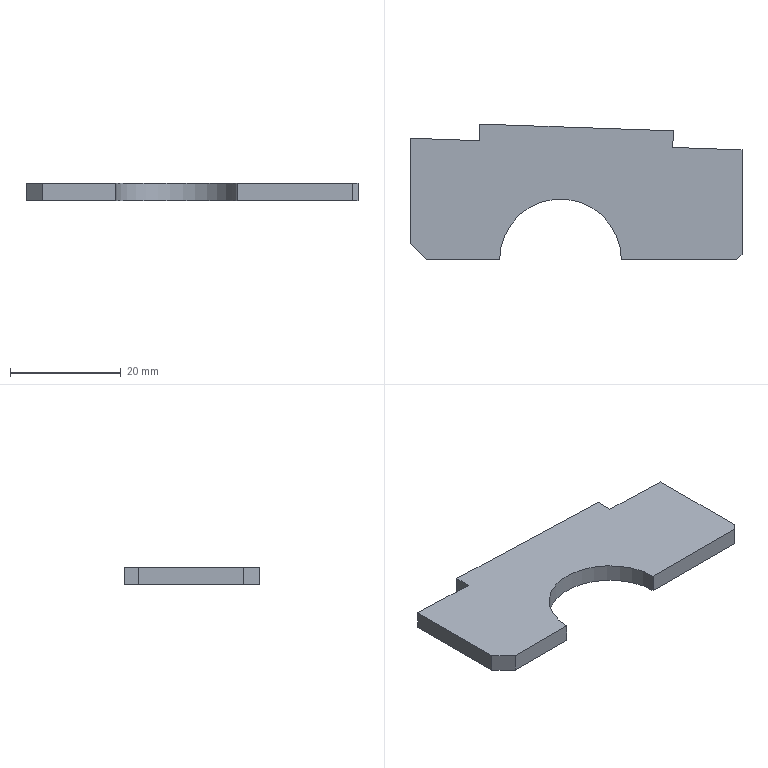Part | SolidWorks | features FlatPattern 1, SMBaseFlange 1, SheetMetal 1 | 1 solid | 14 faces | box 60 x 24.545 x 3.2 mm | volume 3731 mm3 | plane 13 | cylinder 1 | commonest cylinder face diameters 22 x1
STEP:
#1=CARTESIAN_POINT('',(-504.444,-212.712,0.));
#2=VERTEX_POINT('',#1);
#3=CARTESIAN_POINT('',(-501.444,-215.712,0.));
#4=VERTEX_POINT('',#3);
#5=CARTESIAN_POINT('',(-504.444,-212.712,0.));
#6=DIRECTION('',(0.7071,-0.7071,0.));
#7=VECTOR('',#6,1000.);
#8=LINE('',#5,#7);
#9=EDGE_CURVE('',#2,#4,#8,.T.);
#10=ORIENTED_EDGE('',*,*,#9,.T.);
#11=CARTESIAN_POINT('',(-501.444,-215.712,3.2));
#12=VERTEX_POINT('',#11);
#13=CARTESIAN_POINT('',(-501.444,-215.712,3.2));
#14=DIRECTION('',(0.,0.,-1.));
#15=VECTOR('',#14,1000.);
#16=LINE('',#13,#15);
#17=EDGE_CURVE('',#12,#4,#16,.T.);
#18=ORIENTED_EDGE('',*,*,#17,.F.);
#19=CARTESIAN_POINT('',(-504.444,-212.712,3.2));
#20=VERTEX_POINT('',#19);
#21=CARTESIAN_POINT('',(-504.444,-212.712,3.2));
#22=DIRECTION('',(0.7071,-0.7071,0.));
#23=VECTOR('',#22,1000.);
#24=LINE('',#21,#23);
#25=EDGE_CURVE('',#20,#12,#24,.T.);
#26=ORIENTED_EDGE('',*,*,#25,.F.);
#27=CARTESIAN_POINT('',(-504.444,-212.712,3.2));
#28=DIRECTION('',(0.,0.,-1.));
#29=VECTOR('',#28,1000.);
#30=LINE('',#27,#29);
#31=EDGE_CURVE('',#20,#2,#30,.T.);
#32=ORIENTED_EDGE('',*,*,#31,.T.);
#33=EDGE_LOOP('',(#10,#18,#26,#32));
#34=FACE_OUTER_BOUND('',#33,.T.);
#35=CARTESIAN_POINT('',(-504.444,-212.712,3.2));
#36=DIRECTION('',(0.7071,0.7071,0.));
#37=DIRECTION('',(-0.7071,0.7071,0.));
#38=AXIS2_PLACEMENT_3D('',#35,#36,#37);
#39=PLANE('',#38);
#40=ADVANCED_FACE('',(#34),#39,.F.);
#41=CARTESIAN_POINT('',(-488.244,-215.712,0.));
#42=VERTEX_POINT('',#41);
#43=CARTESIAN_POINT('',(-501.444,-215.712,0.));
#44=DIRECTION('',(1.,0.,0.));
#45=VECTOR('',#44,1000.);
#46=LINE('',#43,#45);
#47=EDGE_CURVE('',#4,#42,#46,.T.);
#48=ORIENTED_EDGE('',*,*,#47,.T.);
#49=CARTESIAN_POINT('',(-488.244,-215.712,3.2));
#50=VERTEX_POINT('',#49);
#51=CARTESIAN_POINT('',(-488.244,-215.712,3.2));
#52=DIRECTION('',(0.,0.,-1.));
#53=VECTOR('',#52,1000.);
#54=LINE('',#51,#53);
#55=EDGE_CURVE('',#50,#42,#54,.T.);
#56=ORIENTED_EDGE('',*,*,#55,.F.);
#57=CARTESIAN_POINT('',(-501.444,-215.712,3.2));
#58=DIRECTION('',(1.,0.,0.));
#59=VECTOR('',#58,1000.);
#60=LINE('',#57,#59);
#61=EDGE_CURVE('',#12,#50,#60,.T.);
#62=ORIENTED_EDGE('',*,*,#61,.F.);
#63=ORIENTED_EDGE('',*,*,#17,.T.);
#64=EDGE_LOOP('',(#48,#56,#62,#63));
#65=FACE_OUTER_BOUND('',#64,.T.);
#66=CARTESIAN_POINT('',(-501.444,-215.712,3.2));
#67=DIRECTION('',(0.,1.,0.));
#68=DIRECTION('',(0.,0.,1.));
#69=AXIS2_PLACEMENT_3D('',#66,#67,#68);
#70=PLANE('',#69);
#71=ADVANCED_FACE('',(#65),#70,.F.);
#72=CARTESIAN_POINT('',(-466.244,-215.712,0.));
#73=VERTEX_POINT('',#72);
#74=CARTESIAN_POINT('',(-477.244,-215.712,0.));
#75=DIRECTION('',(0.,0.,-1.));
#76=DIRECTION('',(1.,0.,0.));
#77=AXIS2_PLACEMENT_3D('',#74,#75,#76);
#78=CIRCLE('',#77,11.);
#79=EDGE_CURVE('',#42,#73,#78,.T.);
#80=ORIENTED_EDGE('',*,*,#79,.T.);
#81=CARTESIAN_POINT('',(-466.244,-215.712,3.2));
#82=VERTEX_POINT('',#81);
#83=CARTESIAN_POINT('',(-466.244,-215.712,3.2));
#84=DIRECTION('',(0.,0.,-1.));
#85=VECTOR('',#84,1000.);
#86=LINE('',#83,#85);
#87=EDGE_CURVE('',#82,#73,#86,.T.);
#88=ORIENTED_EDGE('',*,*,#87,.F.);
#89=CARTESIAN_POINT('',(-477.244,-215.712,3.2));
#90=DIRECTION('',(0.,0.,-1.));
#91=DIRECTION('',(1.,0.,0.));
#92=AXIS2_PLACEMENT_3D('',#89,#90,#91);
#93=CIRCLE('',#92,11.);
#94=EDGE_CURVE('',#50,#82,#93,.T.);
#95=ORIENTED_EDGE('',*,*,#94,.F.);
#96=ORIENTED_EDGE('',*,*,#55,.T.);
#97=EDGE_LOOP('',(#80,#88,#95,#96));
#98=FACE_OUTER_BOUND('',#97,.T.);
#99=CARTESIAN_POINT('',(-477.244,-215.712,3.2));
#100=DIRECTION('',(0.,0.,-1.));
#101=DIRECTION('',(-1.,0.,0.));
#102=AXIS2_PLACEMENT_3D('',#99,#100,#101);
#103=CYLINDRICAL_SURFACE('',#102,11.);
#104=ADVANCED_FACE('',(#98),#103,.F.);
#105=CARTESIAN_POINT('',(-445.444,-215.712,0.));
#106=VERTEX_POINT('',#105);
#107=CARTESIAN_POINT('',(-466.244,-215.712,0.));
#108=DIRECTION('',(1.,0.,0.));
#109=VECTOR('',#108,1000.);
#110=LINE('',#107,#109);
#111=EDGE_CURVE('',#73,#106,#110,.T.);
#112=ORIENTED_EDGE('',*,*,#111,.T.);
#113=CARTESIAN_POINT('',(-445.444,-215.712,3.2));
#114=VERTEX_POINT('',#113);
#115=CARTESIAN_POINT('',(-445.444,-215.712,3.2));
#116=DIRECTION('',(0.,0.,-1.));
#117=VECTOR('',#116,1000.);
#118=LINE('',#115,#117);
#119=EDGE_CURVE('',#114,#106,#118,.T.);
#120=ORIENTED_EDGE('',*,*,#119,.F.);
#121=CARTESIAN_POINT('',(-466.244,-215.712,3.2));
#122=DIRECTION('',(1.,0.,0.));
#123=VECTOR('',#122,1000.);
#124=LINE('',#121,#123);
#125=EDGE_CURVE('',#82,#114,#124,.T.);
#126=ORIENTED_EDGE('',*,*,#125,.F.);
#127=ORIENTED_EDGE('',*,*,#87,.T.);
#128=EDGE_LOOP('',(#112,#120,#126,#127));
#129=FACE_OUTER_BOUND('',#128,.T.);
#130=CARTESIAN_POINT('',(-466.244,-215.712,3.2));
#131=DIRECTION('',(0.,1.,0.));
#132=DIRECTION('',(0.,0.,1.));
#133=AXIS2_PLACEMENT_3D('',#130,#131,#132);
#134=PLANE('',#133);
#135=ADVANCED_FACE('',(#129),#134,.F.);
#136=CARTESIAN_POINT('',(-444.444,-214.712,0.));
#137=VERTEX_POINT('',#136);
#138=CARTESIAN_POINT('',(-445.444,-215.712,0.));
#139=DIRECTION('',(0.7071,0.7071,0.));
#140=VECTOR('',#139,1000.);
#141=LINE('',#138,#140);
#142=EDGE_CURVE('',#106,#137,#141,.T.);
#143=ORIENTED_EDGE('',*,*,#142,.T.);
#144=CARTESIAN_POINT('',(-444.444,-214.712,3.2));
#145=VERTEX_POINT('',#144);
#146=CARTESIAN_POINT('',(-444.444,-214.712,3.2));
#147=DIRECTION('',(0.,0.,-1.));
#148=VECTOR('',#147,1000.);
#149=LINE('',#146,#148);
#150=EDGE_CURVE('',#145,#137,#149,.T.);
#151=ORIENTED_EDGE('',*,*,#150,.F.);
#152=CARTESIAN_POINT('',(-445.444,-215.712,3.2));
#153=DIRECTION('',(0.7071,0.7071,0.));
#154=VECTOR('',#153,1000.);
#155=LINE('',#152,#154);
#156=EDGE_CURVE('',#114,#145,#155,.T.);
#157=ORIENTED_EDGE('',*,*,#156,.F.);
#158=ORIENTED_EDGE('',*,*,#119,.T.);
#159=EDGE_LOOP('',(#143,#151,#157,#158));
#160=FACE_OUTER_BOUND('',#159,.T.);
#161=CARTESIAN_POINT('',(-445.444,-215.712,3.2));
#162=DIRECTION('',(-0.7071,0.7071,0.));
#163=DIRECTION('',(-0.7071,-0.7071,0.));
#164=AXIS2_PLACEMENT_3D('',#161,#162,#163);
#165=PLANE('',#164);
#166=ADVANCED_FACE('',(#160),#165,.F.);
#167=CARTESIAN_POINT('',(-444.444,-195.825,0.));
#168=VERTEX_POINT('',#167);
#169=CARTESIAN_POINT('',(-444.444,-214.712,0.));
#170=DIRECTION('',(0.,1.,0.));
#171=VECTOR('',#170,1000.);
#172=LINE('',#169,#171);
#173=EDGE_CURVE('',#137,#168,#172,.T.);
#174=ORIENTED_EDGE('',*,*,#173,.T.);
#175=CARTESIAN_POINT('',(-444.444,-195.825,3.2));
#176=VERTEX_POINT('',#175);
#177=CARTESIAN_POINT('',(-444.444,-195.825,3.2));
#178=DIRECTION('',(0.,0.,-1.));
#179=VECTOR('',#178,1000.);
#180=LINE('',#177,#179);
#181=EDGE_CURVE('',#176,#168,#180,.T.);
#182=ORIENTED_EDGE('',*,*,#181,.F.);
#183=CARTESIAN_POINT('',(-444.444,-214.712,3.2));
#184=DIRECTION('',(0.,1.,0.));
#185=VECTOR('',#184,1000.);
#186=LINE('',#183,#185);
#187=EDGE_CURVE('',#145,#176,#186,.T.);
#188=ORIENTED_EDGE('',*,*,#187,.F.);
#189=ORIENTED_EDGE('',*,*,#150,.T.);
#190=EDGE_LOOP('',(#174,#182,#188,#189));
#191=FACE_OUTER_BOUND('',#190,.T.);
#192=CARTESIAN_POINT('',(-444.444,-214.712,3.2));
#193=DIRECTION('',(-1.,0.,0.));
#194=DIRECTION('',(0.,0.,1.));
#195=AXIS2_PLACEMENT_3D('',#192,#193,#194);
#196=PLANE('',#195);
#197=ADVANCED_FACE('',(#191),#196,.F.);
#198=CARTESIAN_POINT('',(-456.954,-195.388,0.));
#199=VERTEX_POINT('',#198);
#200=CARTESIAN_POINT('',(-444.444,-195.825,0.));
#201=DIRECTION('',(-0.9994,0.0349,0.));
#202=VECTOR('',#201,1000.);
#203=LINE('',#200,#202);
#204=EDGE_CURVE('',#168,#199,#203,.T.);
#205=ORIENTED_EDGE('',*,*,#204,.T.);
#206=CARTESIAN_POINT('',(-456.954,-195.388,3.2));
#207=VERTEX_POINT('',#206);
#208=CARTESIAN_POINT('',(-456.954,-195.388,3.2));
#209=DIRECTION('',(0.,0.,-1.));
#210=VECTOR('',#209,1000.);
#211=LINE('',#208,#210);
#212=EDGE_CURVE('',#207,#199,#211,.T.);
#213=ORIENTED_EDGE('',*,*,#212,.F.);
#214=CARTESIAN_POINT('',(-444.444,-195.825,3.2));
#215=DIRECTION('',(-0.9994,0.0349,0.));
#216=VECTOR('',#215,1000.);
#217=LINE('',#214,#216);
#218=EDGE_CURVE('',#176,#207,#217,.T.);
#219=ORIENTED_EDGE('',*,*,#218,.F.);
#220=ORIENTED_EDGE('',*,*,#181,.T.);
#221=EDGE_LOOP('',(#205,#213,#219,#220));
#222=FACE_OUTER_BOUND('',#221,.T.);
#223=CARTESIAN_POINT('',(-444.444,-195.825,3.2));
#224=DIRECTION('',(-0.0349,-0.9994,0.));
#225=DIRECTION('',(0.9994,-0.0349,0.));
#226=AXIS2_PLACEMENT_3D('',#223,#224,#225);
#227=PLANE('',#226);
#228=ADVANCED_FACE('',(#222),#227,.F.);
#229=CARTESIAN_POINT('',(-456.85,-192.388,0.));
#230=VERTEX_POINT('',#229);
#231=CARTESIAN_POINT('',(-456.954,-195.388,0.));
#232=DIRECTION('',(0.0349,0.9994,0.));
#233=VECTOR('',#232,1000.);
#234=LINE('',#231,#233);
#235=EDGE_CURVE('',#199,#230,#234,.T.);
#236=ORIENTED_EDGE('',*,*,#235,.T.);
#237=CARTESIAN_POINT('',(-456.85,-192.388,3.2));
#238=VERTEX_POINT('',#237);
#239=CARTESIAN_POINT('',(-456.85,-192.388,3.2));
#240=DIRECTION('',(0.,0.,-1.));
#241=VECTOR('',#240,1000.);
#242=LINE('',#239,#241);
#243=EDGE_CURVE('',#238,#230,#242,.T.);
#244=ORIENTED_EDGE('',*,*,#243,.F.);
#245=CARTESIAN_POINT('',(-456.954,-195.388,3.2));
#246=DIRECTION('',(0.0349,0.9994,0.));
#247=VECTOR('',#246,1000.);
#248=LINE('',#245,#247);
#249=EDGE_CURVE('',#207,#238,#248,.T.);
#250=ORIENTED_EDGE('',*,*,#249,.F.);
#251=ORIENTED_EDGE('',*,*,#212,.T.);
#252=EDGE_LOOP('',(#236,#244,#250,#251));
#253=FACE_OUTER_BOUND('',#252,.T.);
#254=CARTESIAN_POINT('',(-456.954,-195.388,3.2));
#255=DIRECTION('',(-0.9994,0.0349,0.));
#256=DIRECTION('',(-0.0349,-0.9994,0.));
#257=AXIS2_PLACEMENT_3D('',#254,#255,#256);
#258=PLANE('',#257);
#259=ADVANCED_FACE('',(#253),#258,.F.);
#260=CARTESIAN_POINT('',(-491.828,-191.167,0.));
#261=VERTEX_POINT('',#260);
#262=CARTESIAN_POINT('',(-456.85,-192.388,0.));
#263=DIRECTION('',(-0.9994,0.0349,0.));
#264=VECTOR('',#263,1000.);
#265=LINE('',#262,#264);
#266=EDGE_CURVE('',#230,#261,#265,.T.);
#267=ORIENTED_EDGE('',*,*,#266,.T.);
#268=CARTESIAN_POINT('',(-491.828,-191.167,3.2));
#269=VERTEX_POINT('',#268);
#270=CARTESIAN_POINT('',(-491.828,-191.167,3.2));
#271=DIRECTION('',(0.,0.,-1.));
#272=VECTOR('',#271,1000.);
#273=LINE('',#270,#272);
#274=EDGE_CURVE('',#269,#261,#273,.T.);
#275=ORIENTED_EDGE('',*,*,#274,.F.);
#276=CARTESIAN_POINT('',(-456.85,-192.388,3.2));
#277=DIRECTION('',(-0.9994,0.0349,0.));
#278=VECTOR('',#277,1000.);
#279=LINE('',#276,#278);
#280=EDGE_CURVE('',#238,#269,#279,.T.);
#281=ORIENTED_EDGE('',*,*,#280,.F.);
#282=ORIENTED_EDGE('',*,*,#243,.T.);
#283=EDGE_LOOP('',(#267,#275,#281,#282));
#284=FACE_OUTER_BOUND('',#283,.T.);
#285=CARTESIAN_POINT('',(-456.85,-192.388,3.2));
#286=DIRECTION('',(-0.0349,-0.9994,0.));
#287=DIRECTION('',(0.9994,-0.0349,0.));
#288=AXIS2_PLACEMENT_3D('',#285,#286,#287);
#289=PLANE('',#288);
#290=ADVANCED_FACE('',(#284),#289,.F.);
#291=CARTESIAN_POINT('',(-491.933,-194.167,0.));
#292=VERTEX_POINT('',#291);
#293=CARTESIAN_POINT('',(-491.828,-191.167,0.));
#294=DIRECTION('',(-0.0349,-0.9994,0.));
#295=VECTOR('',#294,1000.);
#296=LINE('',#293,#295);
#297=EDGE_CURVE('',#261,#292,#296,.T.);
#298=ORIENTED_EDGE('',*,*,#297,.T.);
#299=CARTESIAN_POINT('',(-491.933,-194.167,3.2));
#300=VERTEX_POINT('',#299);
#301=CARTESIAN_POINT('',(-491.933,-194.167,3.2));
#302=DIRECTION('',(0.,0.,-1.));
#303=VECTOR('',#302,1000.);
#304=LINE('',#301,#303);
#305=EDGE_CURVE('',#300,#292,#304,.T.);
#306=ORIENTED_EDGE('',*,*,#305,.F.);
#307=CARTESIAN_POINT('',(-491.828,-191.167,3.2));
#308=DIRECTION('',(-0.0349,-0.9994,0.));
#309=VECTOR('',#308,1000.);
#310=LINE('',#307,#309);
#311=EDGE_CURVE('',#269,#300,#310,.T.);
#312=ORIENTED_EDGE('',*,*,#311,.F.);
#313=ORIENTED_EDGE('',*,*,#274,.T.);
#314=EDGE_LOOP('',(#298,#306,#312,#313));
#315=FACE_OUTER_BOUND('',#314,.T.);
#316=CARTESIAN_POINT('',(-491.828,-191.167,3.2));
#317=DIRECTION('',(0.9994,-0.0349,0.));
#318=DIRECTION('',(0.0349,0.9994,0.));
#319=AXIS2_PLACEMENT_3D('',#316,#317,#318);
#320=PLANE('',#319);
#321=ADVANCED_FACE('',(#315),#320,.F.);
#322=CARTESIAN_POINT('',(-504.444,-193.73,0.));
#323=VERTEX_POINT('',#322);
#324=CARTESIAN_POINT('',(-491.933,-194.167,0.));
#325=DIRECTION('',(-0.9994,0.0349,0.));
#326=VECTOR('',#325,1000.);
#327=LINE('',#324,#326);
#328=EDGE_CURVE('',#292,#323,#327,.T.);
#329=ORIENTED_EDGE('',*,*,#328,.T.);
#330=CARTESIAN_POINT('',(-504.444,-193.73,3.2));
#331=VERTEX_POINT('',#330);
#332=CARTESIAN_POINT('',(-504.444,-193.73,3.2));
#333=DIRECTION('',(0.,0.,-1.));
#334=VECTOR('',#333,1000.);
#335=LINE('',#332,#334);
#336=EDGE_CURVE('',#331,#323,#335,.T.);
#337=ORIENTED_EDGE('',*,*,#336,.F.);
#338=CARTESIAN_POINT('',(-491.933,-194.167,3.2));
#339=DIRECTION('',(-0.9994,0.0349,0.));
#340=VECTOR('',#339,1000.);
#341=LINE('',#338,#340);
#342=EDGE_CURVE('',#300,#331,#341,.T.);
#343=ORIENTED_EDGE('',*,*,#342,.F.);
#344=ORIENTED_EDGE('',*,*,#305,.T.);
#345=EDGE_LOOP('',(#329,#337,#343,#344));
#346=FACE_OUTER_BOUND('',#345,.T.);
#347=CARTESIAN_POINT('',(-491.933,-194.167,3.2));
#348=DIRECTION('',(-0.0349,-0.9994,0.));
#349=DIRECTION('',(0.9994,-0.0349,0.));
#350=AXIS2_PLACEMENT_3D('',#347,#348,#349);
#351=PLANE('',#350);
#352=ADVANCED_FACE('',(#346),#351,.F.);
#353=CARTESIAN_POINT('',(-504.444,-212.712,0.));
#354=DIRECTION('',(0.,-1.,0.));
#355=VECTOR('',#354,1000.);
#356=LINE('',#353,#355);
#357=EDGE_CURVE('',#323,#2,#356,.T.);
#358=ORIENTED_EDGE('',*,*,#357,.T.);
#359=ORIENTED_EDGE('',*,*,#31,.F.);
#360=CARTESIAN_POINT('',(-504.444,-212.712,3.2));
#361=DIRECTION('',(0.,-1.,0.));
#362=VECTOR('',#361,1000.);
#363=LINE('',#360,#362);
#364=EDGE_CURVE('',#331,#20,#363,.T.);
#365=ORIENTED_EDGE('',*,*,#364,.F.);
#366=ORIENTED_EDGE('',*,*,#336,.T.);
#367=EDGE_LOOP('',(#358,#359,#365,#366));
#368=FACE_OUTER_BOUND('',#367,.T.);
#369=CARTESIAN_POINT('',(-504.444,-212.712,3.2));
#370=DIRECTION('',(1.,0.,0.));
#371=DIRECTION('',(0.,0.,-1.));
#372=AXIS2_PLACEMENT_3D('',#369,#370,#371);
#373=PLANE('',#372);
#374=ADVANCED_FACE('',(#368),#373,.F.);
#375=ORIENTED_EDGE('',*,*,#25,.T.);
#376=ORIENTED_EDGE('',*,*,#61,.T.);
#377=ORIENTED_EDGE('',*,*,#94,.T.);
#378=ORIENTED_EDGE('',*,*,#125,.T.);
#379=ORIENTED_EDGE('',*,*,#156,.T.);
#380=ORIENTED_EDGE('',*,*,#187,.T.);
#381=ORIENTED_EDGE('',*,*,#218,.T.);
#382=ORIENTED_EDGE('',*,*,#249,.T.);
#383=ORIENTED_EDGE('',*,*,#280,.T.);
#384=ORIENTED_EDGE('',*,*,#311,.T.);
#385=ORIENTED_EDGE('',*,*,#342,.T.);
#386=ORIENTED_EDGE('',*,*,#364,.T.);
#387=EDGE_LOOP('',(#375,#376,#377,#378,#379,#380,#381,#382,#383,#384,#385,#386));
#388=FACE_OUTER_BOUND('',#387,.T.);
#389=CARTESIAN_POINT('',(-477.244,-215.712,3.2));
#390=DIRECTION('',(0.,0.,1.));
#391=DIRECTION('',(1.,0.,0.));
#392=AXIS2_PLACEMENT_3D('',#389,#390,#391);
#393=PLANE('',#392);
#394=ADVANCED_FACE('',(#388),#393,.T.);
#395=ORIENTED_EDGE('',*,*,#9,.F.);
#396=ORIENTED_EDGE('',*,*,#357,.F.);
#397=ORIENTED_EDGE('',*,*,#328,.F.);
#398=ORIENTED_EDGE('',*,*,#297,.F.);
#399=ORIENTED_EDGE('',*,*,#266,.F.);
#400=ORIENTED_EDGE('',*,*,#235,.F.);
#401=ORIENTED_EDGE('',*,*,#204,.F.);
#402=ORIENTED_EDGE('',*,*,#173,.F.);
#403=ORIENTED_EDGE('',*,*,#142,.F.);
#404=ORIENTED_EDGE('',*,*,#111,.F.);
#405=ORIENTED_EDGE('',*,*,#79,.F.);
#406=ORIENTED_EDGE('',*,*,#47,.F.);
#407=EDGE_LOOP('',(#395,#396,#397,#398,#399,#400,#401,#402,#403,#404,#405,#406));
#408=FACE_OUTER_BOUND('',#407,.T.);
#409=CARTESIAN_POINT('',(-477.244,-215.712,0.));
#410=DIRECTION('',(0.,0.,1.));
#411=DIRECTION('',(1.,0.,0.));
#412=AXIS2_PLACEMENT_3D('',#409,#410,#411);
#413=PLANE('',#412);
#414=ADVANCED_FACE('',(#408),#413,.F.);
#415=CLOSED_SHELL('',(#40,#71,#104,#135,#166,#197,#228,#259,#290,#321,#352,#374,#394,#414));
#416=MANIFOLD_SOLID_BREP('',#415);
#417=CARTESIAN_POINT('',(0.,0.,0.));
#418=DIRECTION('',(0.,0.,1.));
#419=DIRECTION('',(1.,0.,0.));
#420=AXIS2_PLACEMENT_3D('',#417,#418,#419);
#421=(LENGTH_UNIT()NAMED_UNIT(*)SI_UNIT(.MILLI.,.METRE.));
#422=UNCERTAINTY_MEASURE_WITH_UNIT(LENGTH_MEASURE(0.00001),#421,'','');
#423=(NAMED_UNIT(*)PLANE_ANGLE_UNIT()SI_UNIT($,.RADIAN.));
#424=(NAMED_UNIT(*)SI_UNIT($,.STERADIAN.)SOLID_ANGLE_UNIT());
#425=(GEOMETRIC_REPRESENTATION_CONTEXT(3)GLOBAL_UNCERTAINTY_ASSIGNED_CONTEXT((#422))GLOBAL_UNIT_ASSIGNED_CONTEXT((#421,#423,#424))REPRESENTATION_CONTEXT('',''));
#426=ADVANCED_BREP_SHAPE_REPRESENTATION('',(#416,#420),#425);